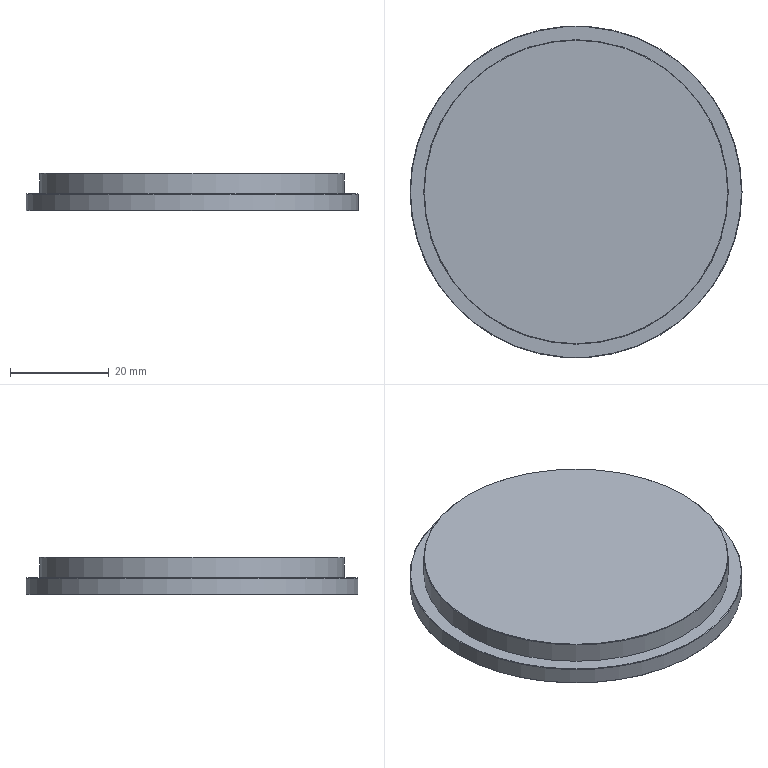Part | NX | features CHAMFER 4, DATUM_CSYS 4, EXTRUDE 3, SKETCH 3, DATUM_PLANE 1 | 1 solid | 11 faces | box 67.2 x 67.2 x 7.62 mm | volume 18147 mm3 | plane 4 | cone 4 | cylinder 3 | commonest cylinder face diameters 49.48 x1 61.62 x1 67.2 x1
STEP:
#1=CARTESIAN_POINT('',(33.6,0.,0.1));
#2=VERTEX_POINT('',#1);
#3=CARTESIAN_POINT('',(0.,0.,0.1));
#4=DIRECTION('',(0.,0.,1.));
#5=DIRECTION('',(1.,0.,0.));
#6=AXIS2_PLACEMENT_3D('',#3,#4,#5);
#7=CIRCLE('',#6,33.6);
#8=EDGE_CURVE('',#2,#2,#7,.T.);
#9=ORIENTED_EDGE('',*,*,#8,.T.);
#10=EDGE_LOOP('',(#9));
#11=FACE_BOUND('',#10,.T.);
#12=CARTESIAN_POINT('',(33.6,0.,3.38));
#13=VERTEX_POINT('',#12);
#14=CARTESIAN_POINT('',(0.,0.,3.38));
#15=DIRECTION('',(0.,0.,1.));
#16=DIRECTION('',(1.,0.,0.));
#17=AXIS2_PLACEMENT_3D('',#14,#15,#16);
#18=CIRCLE('',#17,33.6);
#19=EDGE_CURVE('',#13,#13,#18,.F.);
#20=ORIENTED_EDGE('',*,*,#19,.T.);
#21=EDGE_LOOP('',(#20));
#22=FACE_BOUND('',#21,.T.);
#23=CARTESIAN_POINT('',(0.,0.,7.62));
#24=DIRECTION('',(0.,0.,-1.));
#25=DIRECTION('',(-1.,0.,0.));
#26=AXIS2_PLACEMENT_3D('',#23,#24,#25);
#27=CYLINDRICAL_SURFACE('',#26,33.6);
#28=ADVANCED_FACE('',(#11,#22),#27,.T.);
#29=CARTESIAN_POINT('',(24.84,0.,0.));
#30=VERTEX_POINT('',#29);
#31=CARTESIAN_POINT('',(0.,0.,0.));
#32=DIRECTION('',(0.,0.,1.));
#33=DIRECTION('',(1.,0.,0.));
#34=AXIS2_PLACEMENT_3D('',#31,#32,#33);
#35=CIRCLE('',#34,24.84);
#36=EDGE_CURVE('',#30,#30,#35,.T.);
#37=ORIENTED_EDGE('',*,*,#36,.T.);
#38=EDGE_LOOP('',(#37));
#39=FACE_BOUND('',#38,.T.);
#40=CARTESIAN_POINT('',(33.5,0.,0.));
#41=VERTEX_POINT('',#40);
#42=CARTESIAN_POINT('',(0.,0.,0.));
#43=DIRECTION('',(0.,0.,1.));
#44=DIRECTION('',(1.,0.,0.));
#45=AXIS2_PLACEMENT_3D('',#42,#43,#44);
#46=CIRCLE('',#45,33.5);
#47=EDGE_CURVE('',#41,#41,#46,.F.);
#48=ORIENTED_EDGE('',*,*,#47,.T.);
#49=EDGE_LOOP('',(#48));
#50=FACE_BOUND('',#49,.T.);
#51=CARTESIAN_POINT('',(0.,0.,0.));
#52=DIRECTION('',(0.,0.,1.));
#53=DIRECTION('',(1.,0.,0.));
#54=AXIS2_PLACEMENT_3D('',#51,#52,#53);
#55=PLANE('',#54);
#56=ADVANCED_FACE('',(#39,#50),#55,.F.);
#57=CARTESIAN_POINT('',(24.74,0.,0.1));
#58=VERTEX_POINT('',#57);
#59=CARTESIAN_POINT('',(0.,0.,0.1));
#60=DIRECTION('',(0.,0.,1.));
#61=DIRECTION('',(1.,0.,0.));
#62=AXIS2_PLACEMENT_3D('',#59,#60,#61);
#63=CIRCLE('',#62,24.74);
#64=EDGE_CURVE('',#58,#58,#63,.F.);
#65=ORIENTED_EDGE('',*,*,#64,.T.);
#66=EDGE_LOOP('',(#65));
#67=FACE_BOUND('',#66,.T.);
#68=CARTESIAN_POINT('',(24.74,0.,3.4));
#69=VERTEX_POINT('',#68);
#70=CARTESIAN_POINT('',(0.,0.,3.4));
#71=DIRECTION('',(0.,0.,-1.));
#72=DIRECTION('',(1.,0.,0.));
#73=AXIS2_PLACEMENT_3D('',#70,#71,#72);
#74=CIRCLE('',#73,24.74);
#75=EDGE_CURVE('',#69,#69,#74,.F.);
#76=ORIENTED_EDGE('',*,*,#75,.T.);
#77=EDGE_LOOP('',(#76));
#78=FACE_BOUND('',#77,.T.);
#79=CARTESIAN_POINT('',(0.,0.,3.4));
#80=DIRECTION('',(0.,0.,-1.));
#81=DIRECTION('',(-1.,0.,0.));
#82=AXIS2_PLACEMENT_3D('',#79,#80,#81);
#83=CYLINDRICAL_SURFACE('',#82,24.74);
#84=ADVANCED_FACE('',(#67,#78),#83,.F.);
#85=ORIENTED_EDGE('',*,*,#75,.F.);
#86=EDGE_LOOP('',(#85));
#87=FACE_BOUND('',#86,.T.);
#88=CARTESIAN_POINT('',(0.,0.,3.4));
#89=DIRECTION('',(0.,0.,-1.));
#90=DIRECTION('',(-1.,0.,0.));
#91=AXIS2_PLACEMENT_3D('',#88,#89,#90);
#92=PLANE('',#91);
#93=ADVANCED_FACE('',(#87),#92,.T.);
#94=CARTESIAN_POINT('',(30.81,0.,7.52));
#95=VERTEX_POINT('',#94);
#96=CARTESIAN_POINT('',(0.,0.,7.52));
#97=DIRECTION('',(0.,0.,1.));
#98=DIRECTION('',(1.,0.,0.));
#99=AXIS2_PLACEMENT_3D('',#96,#97,#98);
#100=CIRCLE('',#99,30.81);
#101=EDGE_CURVE('',#95,#95,#100,.F.);
#102=ORIENTED_EDGE('',*,*,#101,.T.);
#103=EDGE_LOOP('',(#102));
#104=FACE_BOUND('',#103,.T.);
#105=CARTESIAN_POINT('',(30.81,0.,3.48));
#106=VERTEX_POINT('',#105);
#107=CARTESIAN_POINT('',(0.,0.,3.48));
#108=DIRECTION('',(0.,0.,1.));
#109=DIRECTION('',(1.,0.,0.));
#110=AXIS2_PLACEMENT_3D('',#107,#108,#109);
#111=CIRCLE('',#110,30.81);
#112=EDGE_CURVE('',#106,#106,#111,.F.);
#113=ORIENTED_EDGE('',*,*,#112,.F.);
#114=EDGE_LOOP('',(#113));
#115=FACE_BOUND('',#114,.T.);
#116=CARTESIAN_POINT('',(0.,0.,3.48));
#117=DIRECTION('',(0.,0.,1.));
#118=DIRECTION('',(1.,0.,0.));
#119=AXIS2_PLACEMENT_3D('',#116,#117,#118);
#120=CYLINDRICAL_SURFACE('',#119,30.81);
#121=ADVANCED_FACE('',(#104,#115),#120,.T.);
#122=CARTESIAN_POINT('',(33.5,0.,3.48));
#123=VERTEX_POINT('',#122);
#124=CARTESIAN_POINT('',(0.,0.,3.48));
#125=DIRECTION('',(0.,0.,1.));
#126=DIRECTION('',(1.,0.,0.));
#127=AXIS2_PLACEMENT_3D('',#124,#125,#126);
#128=CIRCLE('',#127,33.5);
#129=EDGE_CURVE('',#123,#123,#128,.T.);
#130=ORIENTED_EDGE('',*,*,#129,.T.);
#131=EDGE_LOOP('',(#130));
#132=FACE_BOUND('',#131,.T.);
#133=ORIENTED_EDGE('',*,*,#112,.T.);
#134=EDGE_LOOP('',(#133));
#135=FACE_BOUND('',#134,.T.);
#136=CARTESIAN_POINT('',(0.,0.,3.48));
#137=DIRECTION('',(0.,0.,1.));
#138=DIRECTION('',(1.,0.,0.));
#139=AXIS2_PLACEMENT_3D('',#136,#137,#138);
#140=PLANE('',#139);
#141=ADVANCED_FACE('',(#132,#135),#140,.T.);
#142=CARTESIAN_POINT('',(30.71,0.,7.62));
#143=VERTEX_POINT('',#142);
#144=CARTESIAN_POINT('',(0.,0.,7.62));
#145=DIRECTION('',(0.,0.,1.));
#146=DIRECTION('',(1.,0.,0.));
#147=AXIS2_PLACEMENT_3D('',#144,#145,#146);
#148=CIRCLE('',#147,30.71);
#149=EDGE_CURVE('',#143,#143,#148,.T.);
#150=ORIENTED_EDGE('',*,*,#149,.T.);
#151=EDGE_LOOP('',(#150));
#152=FACE_BOUND('',#151,.T.);
#153=CARTESIAN_POINT('',(0.,0.,7.62));
#154=DIRECTION('',(0.,0.,1.));
#155=DIRECTION('',(1.,0.,0.));
#156=AXIS2_PLACEMENT_3D('',#153,#154,#155);
#157=PLANE('',#156);
#158=ADVANCED_FACE('',(#152),#157,.T.);
#159=ORIENTED_EDGE('',*,*,#101,.F.);
#160=EDGE_LOOP('',(#159));
#161=FACE_BOUND('',#160,.T.);
#162=ORIENTED_EDGE('',*,*,#149,.F.);
#163=EDGE_LOOP('',(#162));
#164=FACE_BOUND('',#163,.T.);
#165=CARTESIAN_POINT('',(0.,0.,7.62));
#166=DIRECTION('',(0.,0.,-1.));
#167=DIRECTION('',(-1.,0.,0.));
#168=AXIS2_PLACEMENT_3D('',#165,#166,#167);
#169=CONICAL_SURFACE('',#168,30.71,0.7854);
#170=ADVANCED_FACE('',(#161,#164),#169,.T.);
#171=ORIENTED_EDGE('',*,*,#19,.F.);
#172=EDGE_LOOP('',(#171));
#173=FACE_BOUND('',#172,.T.);
#174=ORIENTED_EDGE('',*,*,#129,.F.);
#175=EDGE_LOOP('',(#174));
#176=FACE_BOUND('',#175,.T.);
#177=CARTESIAN_POINT('',(0.,0.,3.48));
#178=DIRECTION('',(0.,0.,-1.));
#179=DIRECTION('',(-1.,0.,0.));
#180=AXIS2_PLACEMENT_3D('',#177,#178,#179);
#181=CONICAL_SURFACE('',#180,33.5,0.7854);
#182=ADVANCED_FACE('',(#173,#176),#181,.T.);
#183=ORIENTED_EDGE('',*,*,#47,.F.);
#184=EDGE_LOOP('',(#183));
#185=FACE_BOUND('',#184,.T.);
#186=ORIENTED_EDGE('',*,*,#8,.F.);
#187=EDGE_LOOP('',(#186));
#188=FACE_BOUND('',#187,.T.);
#189=CARTESIAN_POINT('',(0.,0.,0.1));
#190=DIRECTION('',(0.,0.,1.));
#191=DIRECTION('',(1.,0.,0.));
#192=AXIS2_PLACEMENT_3D('',#189,#190,#191);
#193=CONICAL_SURFACE('',#192,33.6,0.7854);
#194=ADVANCED_FACE('',(#185,#188),#193,.T.);
#195=ORIENTED_EDGE('',*,*,#36,.F.);
#196=EDGE_LOOP('',(#195));
#197=FACE_BOUND('',#196,.T.);
#198=ORIENTED_EDGE('',*,*,#64,.F.);
#199=EDGE_LOOP('',(#198));
#200=FACE_BOUND('',#199,.T.);
#201=CARTESIAN_POINT('',(0.,0.,0.1));
#202=DIRECTION('',(0.,0.,-1.));
#203=DIRECTION('',(-1.,0.,0.));
#204=AXIS2_PLACEMENT_3D('',#201,#202,#203);
#205=CONICAL_SURFACE('',#204,24.74,0.7854);
#206=ADVANCED_FACE('',(#197,#200),#205,.F.);
#207=CLOSED_SHELL('',(#28,#56,#84,#93,#121,#141,#158,#170,#182,#194,#206));
#208=MANIFOLD_SOLID_BREP('',#207);
#209=(LENGTH_UNIT()NAMED_UNIT(*)SI_UNIT(.MILLI.,.METRE.));
#210=UNCERTAINTY_MEASURE_WITH_UNIT(LENGTH_MEASURE(0.00001),#209,'','');
#211=(NAMED_UNIT(*)PLANE_ANGLE_UNIT()SI_UNIT($,.RADIAN.));
#212=(NAMED_UNIT(*)SI_UNIT($,.STERADIAN.)SOLID_ANGLE_UNIT());
#213=(GEOMETRIC_REPRESENTATION_CONTEXT(3)GLOBAL_UNCERTAINTY_ASSIGNED_CONTEXT((#210))GLOBAL_UNIT_ASSIGNED_CONTEXT((#209,#211,#212))REPRESENTATION_CONTEXT('',''));
#214=ADVANCED_BREP_SHAPE_REPRESENTATION('',(#208),#213);